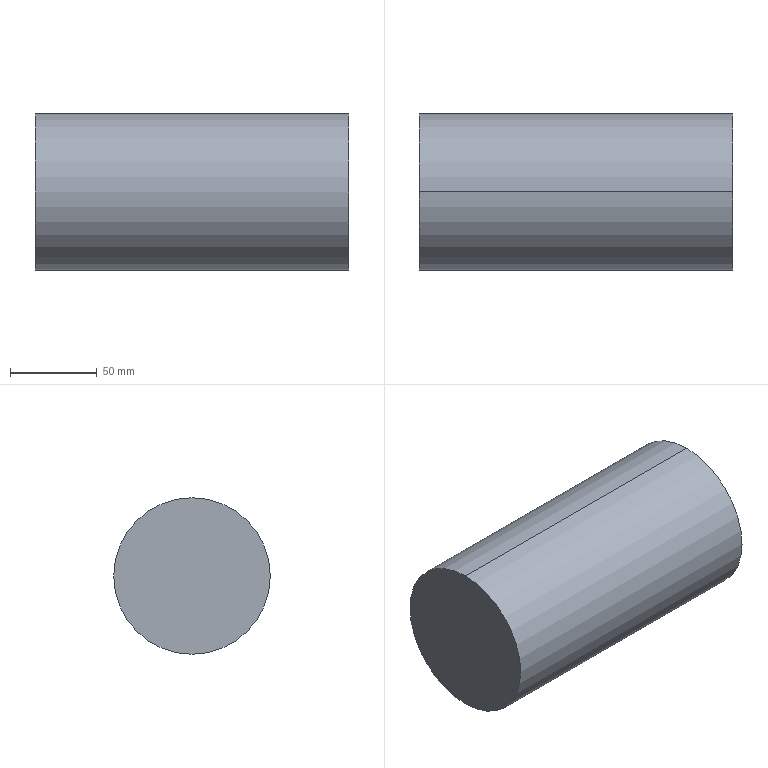Part | NX | 1 solid | 4 faces | box 180 x 90 x 90 mm | volume 1145111 mm3 | cylinder 2 | plane 2 | commonest cylinder face diameters 90 x2
STEP:
#1=CARTESIAN_POINT('',(220.674,199.501,428.798));
#2=VERTEX_POINT('',#1);
#3=CARTESIAN_POINT('',(220.674,199.501,338.798));
#4=VERTEX_POINT('',#3);
#5=CARTESIAN_POINT('',(220.674,199.501,383.798));
#6=DIRECTION('',(-1.,0.,0.));
#7=DIRECTION('',(0.,0.,1.));
#8=AXIS2_PLACEMENT_3D('',#5,#6,#7);
#9=CIRCLE('',#8,45.);
#10=EDGE_CURVE('',#2,#4,#9,.T.);
#11=ORIENTED_EDGE('',*,*,#10,.T.);
#12=CARTESIAN_POINT('',(40.674,199.501,338.798));
#13=VERTEX_POINT('',#12);
#14=CARTESIAN_POINT('',(347.953,199.501,338.798));
#15=DIRECTION('',(-1.,0.,0.));
#16=VECTOR('',#15,1.);
#17=LINE('',#14,#16);
#18=EDGE_CURVE('',#4,#13,#17,.T.);
#19=ORIENTED_EDGE('',*,*,#18,.T.);
#20=CARTESIAN_POINT('',(40.674,199.501,428.798));
#21=VERTEX_POINT('',#20);
#22=CARTESIAN_POINT('',(40.674,199.501,383.798));
#23=DIRECTION('',(1.,0.,0.));
#24=DIRECTION('',(0.,0.,-1.));
#25=AXIS2_PLACEMENT_3D('',#22,#23,#24);
#26=CIRCLE('',#25,45.);
#27=EDGE_CURVE('',#13,#21,#26,.T.);
#28=ORIENTED_EDGE('',*,*,#27,.T.);
#29=CARTESIAN_POINT('',(347.953,199.501,428.798));
#30=DIRECTION('',(1.,0.,0.));
#31=VECTOR('',#30,1.);
#32=LINE('',#29,#31);
#33=EDGE_CURVE('',#21,#2,#32,.T.);
#34=ORIENTED_EDGE('',*,*,#33,.T.);
#35=EDGE_LOOP('',(#11,#19,#28,#34));
#36=FACE_OUTER_BOUND('',#35,.T.);
#37=CARTESIAN_POINT('',(347.953,199.501,383.798));
#38=DIRECTION('',(-1.,0.,0.));
#39=DIRECTION('',(0.,0.,1.));
#40=AXIS2_PLACEMENT_3D('',#37,#38,#39);
#41=CYLINDRICAL_SURFACE('',#40,45.);
#42=ADVANCED_FACE('',(#36),#41,.T.);
#43=CARTESIAN_POINT('',(40.674,199.501,383.798));
#44=DIRECTION('',(1.,0.,0.));
#45=DIRECTION('',(0.,0.,-1.));
#46=AXIS2_PLACEMENT_3D('',#43,#44,#45);
#47=CIRCLE('',#46,45.);
#48=EDGE_CURVE('',#21,#13,#47,.T.);
#49=ORIENTED_EDGE('',*,*,#48,.F.);
#50=ORIENTED_EDGE('',*,*,#27,.F.);
#51=EDGE_LOOP('',(#49,#50));
#52=FACE_OUTER_BOUND('',#51,.T.);
#53=CARTESIAN_POINT('',(40.674,199.501,383.798));
#54=DIRECTION('',(1.,0.,0.));
#55=DIRECTION('',(0.,0.,-1.));
#56=AXIS2_PLACEMENT_3D('',#53,#54,#55);
#57=PLANE('',#56);
#58=ADVANCED_FACE('',(#52),#57,.F.);
#59=ORIENTED_EDGE('',*,*,#18,.F.);
#60=CARTESIAN_POINT('',(220.674,199.501,383.798));
#61=DIRECTION('',(-1.,0.,0.));
#62=DIRECTION('',(0.,0.,1.));
#63=AXIS2_PLACEMENT_3D('',#60,#61,#62);
#64=CIRCLE('',#63,45.);
#65=EDGE_CURVE('',#4,#2,#64,.T.);
#66=ORIENTED_EDGE('',*,*,#65,.T.);
#67=ORIENTED_EDGE('',*,*,#33,.F.);
#68=ORIENTED_EDGE('',*,*,#48,.T.);
#69=EDGE_LOOP('',(#59,#66,#67,#68));
#70=FACE_OUTER_BOUND('',#69,.T.);
#71=CARTESIAN_POINT('',(347.953,199.501,383.798));
#72=DIRECTION('',(-1.,0.,0.));
#73=DIRECTION('',(0.,0.,1.));
#74=AXIS2_PLACEMENT_3D('',#71,#72,#73);
#75=CYLINDRICAL_SURFACE('',#74,45.);
#76=ADVANCED_FACE('',(#70),#75,.T.);
#77=ORIENTED_EDGE('',*,*,#10,.F.);
#78=ORIENTED_EDGE('',*,*,#65,.F.);
#79=EDGE_LOOP('',(#77,#78));
#80=FACE_OUTER_BOUND('',#79,.T.);
#81=CARTESIAN_POINT('',(220.674,-484.499,2185.086));
#82=DIRECTION('',(-1.,0.,0.));
#83=DIRECTION('',(0.,0.,-1.));
#84=AXIS2_PLACEMENT_3D('',#81,#82,#83);
#85=PLANE('',#84);
#86=ADVANCED_FACE('',(#80),#85,.F.);
#87=CLOSED_SHELL('',(#42,#58,#76,#86));
#88=MANIFOLD_SOLID_BREP('',#87);
#89=(LENGTH_UNIT()NAMED_UNIT(*)SI_UNIT(.MILLI.,.METRE.));
#90=UNCERTAINTY_MEASURE_WITH_UNIT(LENGTH_MEASURE(0.00002),#89,'','');
#91=(NAMED_UNIT(*)PLANE_ANGLE_UNIT()SI_UNIT($,.RADIAN.));
#92=PLANE_ANGLE_MEASURE_WITH_UNIT(PLANE_ANGLE_MEASURE(0.01745),#91);
#93=DIMENSIONAL_EXPONENTS(0.,0.,0.,0.,0.,0.,0.);
#94=(CONVERSION_BASED_UNIT('DEGREE',#92)NAMED_UNIT(#93)PLANE_ANGLE_UNIT());
#95=(NAMED_UNIT(*)SI_UNIT($,.STERADIAN.)SOLID_ANGLE_UNIT());
#96=(GEOMETRIC_REPRESENTATION_CONTEXT(3)GLOBAL_UNCERTAINTY_ASSIGNED_CONTEXT((#90))GLOBAL_UNIT_ASSIGNED_CONTEXT((#89,#94,#95))REPRESENTATION_CONTEXT('',''));
#97=ADVANCED_BREP_SHAPE_REPRESENTATION('',(#88),#96);